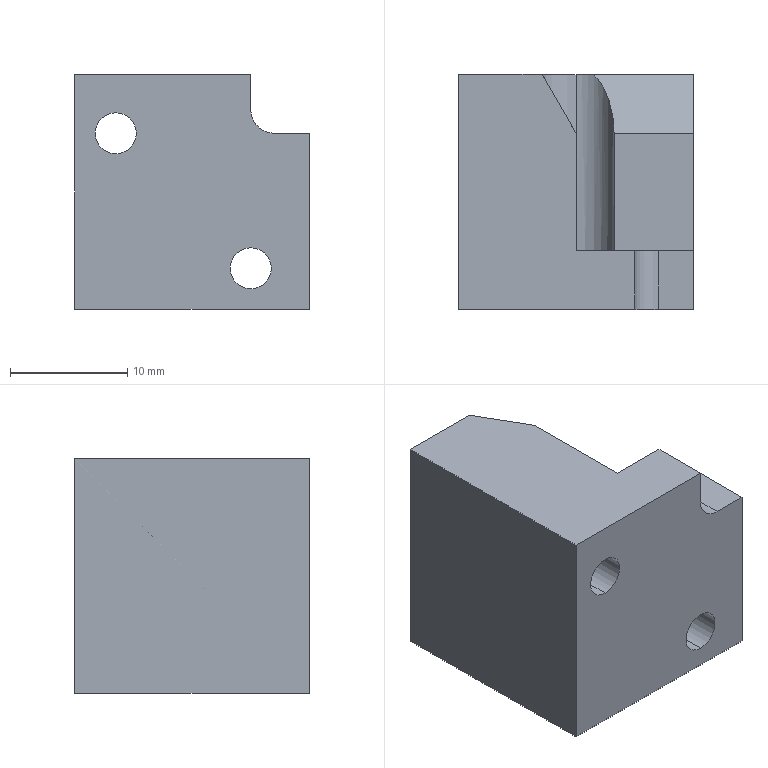Part | STEP file | 0217_017_WGDLJ-20-5-5 | 1 solid | 27 faces | box 20 x 20 x 20 mm | volume 5354 mm3 | plane 16 | cylinder 11 | commonest cylinder face diameters 6.5 x6 3.5 x4 4 x1